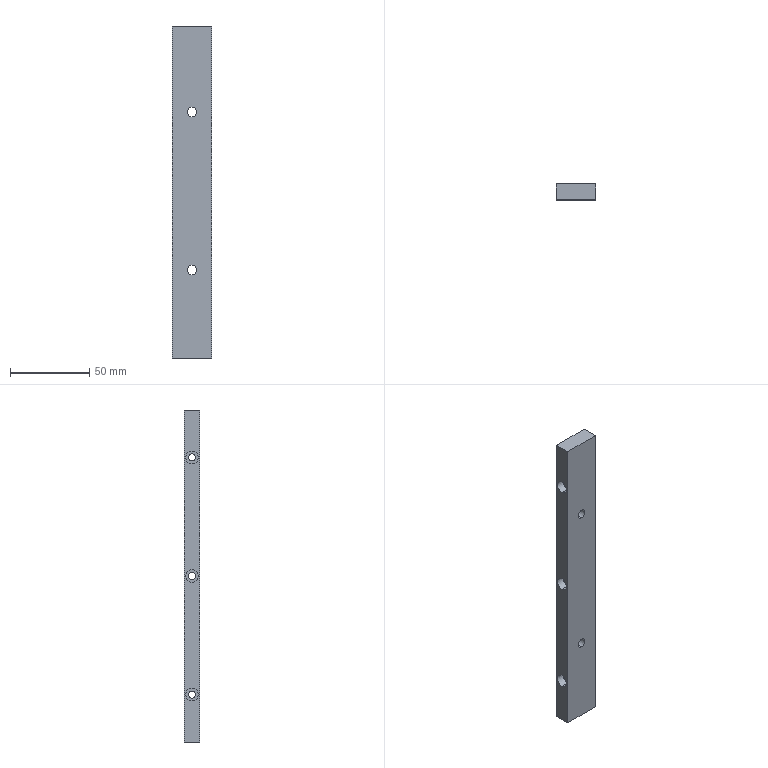Part | SolidWorks | features Extrusion 1, HoleWzd 1, ICE 1 | 1 solid | 25 faces | box 25 x 10 x 210 mm | volume 50226 mm3 | cylinder 16 | plane 9 | commonest cylinder face diameters 4.5 x6 8 x6 6 x4
STEP:
#1=CARTESIAN_POINT('',(0.,5.,-46.436));
#2=VERTEX_POINT('',#1);
#3=CARTESIAN_POINT('',(0.,5.,-52.436));
#4=VERTEX_POINT('',#3);
#5=CARTESIAN_POINT('',(0.,5.,-49.436));
#6=DIRECTION('',(0.,-1.,0.));
#7=DIRECTION('',(0.,0.,-1.));
#8=AXIS2_PLACEMENT_3D('',#5,#6,#7);
#9=CIRCLE('',#8,3.);
#10=EDGE_CURVE('',#2,#4,#9,.T.);
#11=ORIENTED_EDGE('',*,*,#10,.F.);
#12=CARTESIAN_POINT('',(0.,-5.,-46.436));
#13=VERTEX_POINT('',#12);
#14=CARTESIAN_POINT('',(0.,24.,-46.436));
#15=DIRECTION('',(0.,-1.,0.));
#16=VECTOR('',#15,1000.);
#17=LINE('',#14,#16);
#18=EDGE_CURVE('',#2,#13,#17,.T.);
#19=ORIENTED_EDGE('',*,*,#18,.T.);
#20=CARTESIAN_POINT('',(0.,-5.,-52.436));
#21=VERTEX_POINT('',#20);
#22=CARTESIAN_POINT('',(0.,-5.,-49.436));
#23=DIRECTION('',(0.,-1.,0.));
#24=DIRECTION('',(0.,0.,-1.));
#25=AXIS2_PLACEMENT_3D('',#22,#23,#24);
#26=CIRCLE('',#25,3.);
#27=EDGE_CURVE('',#13,#21,#26,.T.);
#28=ORIENTED_EDGE('',*,*,#27,.T.);
#29=CARTESIAN_POINT('',(0.,24.,-52.436));
#30=DIRECTION('',(0.,-1.,0.));
#31=VECTOR('',#30,1000.);
#32=LINE('',#29,#31);
#33=EDGE_CURVE('',#4,#21,#32,.T.);
#34=ORIENTED_EDGE('',*,*,#33,.F.);
#35=EDGE_LOOP('',(#11,#19,#28,#34));
#36=FACE_OUTER_BOUND('',#35,.T.);
#37=CARTESIAN_POINT('',(0.,24.,-49.436));
#38=DIRECTION('',(0.,-1.,0.));
#39=DIRECTION('',(0.,0.,-1.));
#40=AXIS2_PLACEMENT_3D('',#37,#38,#39);
#41=CYLINDRICAL_SURFACE('',#40,3.);
#42=ADVANCED_FACE('',(#36),#41,.F.);
#43=CARTESIAN_POINT('',(0.,5.,53.564));
#44=VERTEX_POINT('',#43);
#45=CARTESIAN_POINT('',(0.,5.,47.564));
#46=VERTEX_POINT('',#45);
#47=CARTESIAN_POINT('',(0.,5.,50.564));
#48=DIRECTION('',(0.,-1.,0.));
#49=DIRECTION('',(0.,0.,-1.));
#50=AXIS2_PLACEMENT_3D('',#47,#48,#49);
#51=CIRCLE('',#50,3.);
#52=EDGE_CURVE('',#44,#46,#51,.T.);
#53=ORIENTED_EDGE('',*,*,#52,.F.);
#54=CARTESIAN_POINT('',(0.,-5.,53.564));
#55=VERTEX_POINT('',#54);
#56=CARTESIAN_POINT('',(0.,24.,53.564));
#57=DIRECTION('',(0.,-1.,0.));
#58=VECTOR('',#57,1000.);
#59=LINE('',#56,#58);
#60=EDGE_CURVE('',#44,#55,#59,.T.);
#61=ORIENTED_EDGE('',*,*,#60,.T.);
#62=CARTESIAN_POINT('',(0.,-5.,47.564));
#63=VERTEX_POINT('',#62);
#64=CARTESIAN_POINT('',(0.,-5.,50.564));
#65=DIRECTION('',(0.,-1.,0.));
#66=DIRECTION('',(0.,0.,-1.));
#67=AXIS2_PLACEMENT_3D('',#64,#65,#66);
#68=CIRCLE('',#67,3.);
#69=EDGE_CURVE('',#55,#63,#68,.T.);
#70=ORIENTED_EDGE('',*,*,#69,.T.);
#71=CARTESIAN_POINT('',(0.,24.,47.564));
#72=DIRECTION('',(0.,-1.,0.));
#73=VECTOR('',#72,1000.);
#74=LINE('',#71,#73);
#75=EDGE_CURVE('',#46,#63,#74,.T.);
#76=ORIENTED_EDGE('',*,*,#75,.F.);
#77=EDGE_LOOP('',(#53,#61,#70,#76));
#78=FACE_OUTER_BOUND('',#77,.T.);
#79=CARTESIAN_POINT('',(0.,24.,50.564));
#80=DIRECTION('',(0.,-1.,0.));
#81=DIRECTION('',(0.,0.,-1.));
#82=AXIS2_PLACEMENT_3D('',#79,#80,#81);
#83=CYLINDRICAL_SURFACE('',#82,3.);
#84=ADVANCED_FACE('',(#78),#83,.F.);
#85=CARTESIAN_POINT('',(-7.5,0.,-4.));
#86=VERTEX_POINT('',#85);
#87=CARTESIAN_POINT('',(-7.5,0.,4.));
#88=VERTEX_POINT('',#87);
#89=CARTESIAN_POINT('',(-7.5,0.,0.));
#90=DIRECTION('',(-1.,0.,0.));
#91=DIRECTION('',(0.,0.,1.));
#92=AXIS2_PLACEMENT_3D('',#89,#90,#91);
#93=CIRCLE('',#92,4.);
#94=EDGE_CURVE('',#86,#88,#93,.T.);
#95=ORIENTED_EDGE('',*,*,#94,.F.);
#96=CARTESIAN_POINT('',(-12.5,0.,-4.));
#97=VERTEX_POINT('',#96);
#98=CARTESIAN_POINT('',(-12.5,0.,-4.));
#99=DIRECTION('',(-1.,0.,0.));
#100=VECTOR('',#99,1000.);
#101=LINE('',#98,#100);
#102=EDGE_CURVE('',#86,#97,#101,.T.);
#103=ORIENTED_EDGE('',*,*,#102,.T.);
#104=CARTESIAN_POINT('',(-12.5,0.,4.));
#105=VERTEX_POINT('',#104);
#106=CARTESIAN_POINT('',(-12.5,0.,0.));
#107=DIRECTION('',(-1.,0.,0.));
#108=DIRECTION('',(0.,0.,1.));
#109=AXIS2_PLACEMENT_3D('',#106,#107,#108);
#110=CIRCLE('',#109,4.);
#111=EDGE_CURVE('',#97,#105,#110,.T.);
#112=ORIENTED_EDGE('',*,*,#111,.T.);
#113=CARTESIAN_POINT('',(-12.5,0.,4.));
#114=DIRECTION('',(-1.,0.,0.));
#115=VECTOR('',#114,1000.);
#116=LINE('',#113,#115);
#117=EDGE_CURVE('',#88,#105,#116,.T.);
#118=ORIENTED_EDGE('',*,*,#117,.F.);
#119=EDGE_LOOP('',(#95,#103,#112,#118));
#120=FACE_OUTER_BOUND('',#119,.T.);
#121=CARTESIAN_POINT('',(-12.5,0.,0.));
#122=DIRECTION('',(-1.,0.,0.));
#123=DIRECTION('',(0.,0.,1.));
#124=AXIS2_PLACEMENT_3D('',#121,#122,#123);
#125=CYLINDRICAL_SURFACE('',#124,4.);
#126=ADVANCED_FACE('',(#120),#125,.F.);
#127=CARTESIAN_POINT('',(12.5,0.,-2.25));
#128=VERTEX_POINT('',#127);
#129=CARTESIAN_POINT('',(12.5,0.,2.25));
#130=VERTEX_POINT('',#129);
#131=CARTESIAN_POINT('',(12.5,0.,0.));
#132=DIRECTION('',(-1.,0.,0.));
#133=DIRECTION('',(0.,0.,1.));
#134=AXIS2_PLACEMENT_3D('',#131,#132,#133);
#135=CIRCLE('',#134,2.25);
#136=EDGE_CURVE('',#128,#130,#135,.T.);
#137=ORIENTED_EDGE('',*,*,#136,.F.);
#138=CARTESIAN_POINT('',(-7.5,0.,-2.25));
#139=VERTEX_POINT('',#138);
#140=CARTESIAN_POINT('',(-12.5,0.,-2.25));
#141=DIRECTION('',(-1.,0.,0.));
#142=VECTOR('',#141,1000.);
#143=LINE('',#140,#142);
#144=EDGE_CURVE('',#128,#139,#143,.T.);
#145=ORIENTED_EDGE('',*,*,#144,.T.);
#146=CARTESIAN_POINT('',(-7.5,0.,2.25));
#147=VERTEX_POINT('',#146);
#148=CARTESIAN_POINT('',(-7.5,0.,0.));
#149=DIRECTION('',(-1.,0.,0.));
#150=DIRECTION('',(0.,0.,1.));
#151=AXIS2_PLACEMENT_3D('',#148,#149,#150);
#152=CIRCLE('',#151,2.25);
#153=EDGE_CURVE('',#139,#147,#152,.T.);
#154=ORIENTED_EDGE('',*,*,#153,.T.);
#155=CARTESIAN_POINT('',(-12.5,0.,2.25));
#156=DIRECTION('',(-1.,0.,0.));
#157=VECTOR('',#156,1000.);
#158=LINE('',#155,#157);
#159=EDGE_CURVE('',#130,#147,#158,.T.);
#160=ORIENTED_EDGE('',*,*,#159,.F.);
#161=EDGE_LOOP('',(#137,#145,#154,#160));
#162=FACE_OUTER_BOUND('',#161,.T.);
#163=CARTESIAN_POINT('',(-12.5,0.,0.));
#164=DIRECTION('',(-1.,0.,0.));
#165=DIRECTION('',(0.,0.,1.));
#166=AXIS2_PLACEMENT_3D('',#163,#164,#165);
#167=CYLINDRICAL_SURFACE('',#166,2.25);
#168=ADVANCED_FACE('',(#162),#167,.F.);
#169=CARTESIAN_POINT('',(-7.5,0.,-79.));
#170=VERTEX_POINT('',#169);
#171=CARTESIAN_POINT('',(-7.5,0.,-71.));
#172=VERTEX_POINT('',#171);
#173=CARTESIAN_POINT('',(-7.5,0.,-75.));
#174=DIRECTION('',(-1.,0.,0.));
#175=DIRECTION('',(0.,0.,1.));
#176=AXIS2_PLACEMENT_3D('',#173,#174,#175);
#177=CIRCLE('',#176,4.);
#178=EDGE_CURVE('',#170,#172,#177,.T.);
#179=ORIENTED_EDGE('',*,*,#178,.F.);
#180=CARTESIAN_POINT('',(-12.5,0.,-79.));
#181=VERTEX_POINT('',#180);
#182=CARTESIAN_POINT('',(-12.5,0.,-79.));
#183=DIRECTION('',(-1.,0.,0.));
#184=VECTOR('',#183,1000.);
#185=LINE('',#182,#184);
#186=EDGE_CURVE('',#170,#181,#185,.T.);
#187=ORIENTED_EDGE('',*,*,#186,.T.);
#188=CARTESIAN_POINT('',(-12.5,0.,-71.));
#189=VERTEX_POINT('',#188);
#190=CARTESIAN_POINT('',(-12.5,0.,-75.));
#191=DIRECTION('',(-1.,0.,0.));
#192=DIRECTION('',(0.,0.,1.));
#193=AXIS2_PLACEMENT_3D('',#190,#191,#192);
#194=CIRCLE('',#193,4.);
#195=EDGE_CURVE('',#181,#189,#194,.T.);
#196=ORIENTED_EDGE('',*,*,#195,.T.);
#197=CARTESIAN_POINT('',(-12.5,0.,-71.));
#198=DIRECTION('',(-1.,0.,0.));
#199=VECTOR('',#198,1000.);
#200=LINE('',#197,#199);
#201=EDGE_CURVE('',#172,#189,#200,.T.);
#202=ORIENTED_EDGE('',*,*,#201,.F.);
#203=EDGE_LOOP('',(#179,#187,#196,#202));
#204=FACE_OUTER_BOUND('',#203,.T.);
#205=CARTESIAN_POINT('',(-12.5,0.,-75.));
#206=DIRECTION('',(-1.,0.,0.));
#207=DIRECTION('',(0.,0.,1.));
#208=AXIS2_PLACEMENT_3D('',#205,#206,#207);
#209=CYLINDRICAL_SURFACE('',#208,4.);
#210=ADVANCED_FACE('',(#204),#209,.F.);
#211=CARTESIAN_POINT('',(12.5,0.,-77.25));
#212=VERTEX_POINT('',#211);
#213=CARTESIAN_POINT('',(12.5,0.,-72.75));
#214=VERTEX_POINT('',#213);
#215=CARTESIAN_POINT('',(12.5,0.,-75.));
#216=DIRECTION('',(-1.,0.,0.));
#217=DIRECTION('',(0.,0.,1.));
#218=AXIS2_PLACEMENT_3D('',#215,#216,#217);
#219=CIRCLE('',#218,2.25);
#220=EDGE_CURVE('',#212,#214,#219,.T.);
#221=ORIENTED_EDGE('',*,*,#220,.F.);
#222=CARTESIAN_POINT('',(-7.5,0.,-77.25));
#223=VERTEX_POINT('',#222);
#224=CARTESIAN_POINT('',(-12.5,0.,-77.25));
#225=DIRECTION('',(-1.,0.,0.));
#226=VECTOR('',#225,1000.);
#227=LINE('',#224,#226);
#228=EDGE_CURVE('',#212,#223,#227,.T.);
#229=ORIENTED_EDGE('',*,*,#228,.T.);
#230=CARTESIAN_POINT('',(-7.5,0.,-72.75));
#231=VERTEX_POINT('',#230);
#232=CARTESIAN_POINT('',(-7.5,0.,-75.));
#233=DIRECTION('',(-1.,0.,0.));
#234=DIRECTION('',(0.,0.,1.));
#235=AXIS2_PLACEMENT_3D('',#232,#233,#234);
#236=CIRCLE('',#235,2.25);
#237=EDGE_CURVE('',#223,#231,#236,.T.);
#238=ORIENTED_EDGE('',*,*,#237,.T.);
#239=CARTESIAN_POINT('',(-12.5,0.,-72.75));
#240=DIRECTION('',(-1.,0.,0.));
#241=VECTOR('',#240,1000.);
#242=LINE('',#239,#241);
#243=EDGE_CURVE('',#214,#231,#242,.T.);
#244=ORIENTED_EDGE('',*,*,#243,.F.);
#245=EDGE_LOOP('',(#221,#229,#238,#244));
#246=FACE_OUTER_BOUND('',#245,.T.);
#247=CARTESIAN_POINT('',(-12.5,0.,-75.));
#248=DIRECTION('',(-1.,0.,0.));
#249=DIRECTION('',(0.,0.,1.));
#250=AXIS2_PLACEMENT_3D('',#247,#248,#249);
#251=CYLINDRICAL_SURFACE('',#250,2.25);
#252=ADVANCED_FACE('',(#246),#251,.F.);
#253=CARTESIAN_POINT('',(-7.5,0.,71.));
#254=VERTEX_POINT('',#253);
#255=CARTESIAN_POINT('',(-7.5,0.,79.));
#256=VERTEX_POINT('',#255);
#257=CARTESIAN_POINT('',(-7.5,0.,75.));
#258=DIRECTION('',(-1.,0.,0.));
#259=DIRECTION('',(0.,0.,1.));
#260=AXIS2_PLACEMENT_3D('',#257,#258,#259);
#261=CIRCLE('',#260,4.);
#262=EDGE_CURVE('',#254,#256,#261,.T.);
#263=ORIENTED_EDGE('',*,*,#262,.F.);
#264=CARTESIAN_POINT('',(-12.5,0.,71.));
#265=VERTEX_POINT('',#264);
#266=CARTESIAN_POINT('',(-12.5,0.,71.));
#267=DIRECTION('',(-1.,0.,0.));
#268=VECTOR('',#267,1000.);
#269=LINE('',#266,#268);
#270=EDGE_CURVE('',#254,#265,#269,.T.);
#271=ORIENTED_EDGE('',*,*,#270,.T.);
#272=CARTESIAN_POINT('',(-12.5,0.,79.));
#273=VERTEX_POINT('',#272);
#274=CARTESIAN_POINT('',(-12.5,0.,75.));
#275=DIRECTION('',(-1.,0.,0.));
#276=DIRECTION('',(0.,0.,1.));
#277=AXIS2_PLACEMENT_3D('',#274,#275,#276);
#278=CIRCLE('',#277,4.);
#279=EDGE_CURVE('',#265,#273,#278,.T.);
#280=ORIENTED_EDGE('',*,*,#279,.T.);
#281=CARTESIAN_POINT('',(-12.5,0.,79.));
#282=DIRECTION('',(-1.,0.,0.));
#283=VECTOR('',#282,1000.);
#284=LINE('',#281,#283);
#285=EDGE_CURVE('',#256,#273,#284,.T.);
#286=ORIENTED_EDGE('',*,*,#285,.F.);
#287=EDGE_LOOP('',(#263,#271,#280,#286));
#288=FACE_OUTER_BOUND('',#287,.T.);
#289=CARTESIAN_POINT('',(-12.5,0.,75.));
#290=DIRECTION('',(-1.,0.,0.));
#291=DIRECTION('',(0.,0.,1.));
#292=AXIS2_PLACEMENT_3D('',#289,#290,#291);
#293=CYLINDRICAL_SURFACE('',#292,4.);
#294=ADVANCED_FACE('',(#288),#293,.F.);
#295=CARTESIAN_POINT('',(12.5,0.,72.75));
#296=VERTEX_POINT('',#295);
#297=CARTESIAN_POINT('',(12.5,0.,77.25));
#298=VERTEX_POINT('',#297);
#299=CARTESIAN_POINT('',(12.5,0.,75.));
#300=DIRECTION('',(-1.,0.,0.));
#301=DIRECTION('',(0.,0.,1.));
#302=AXIS2_PLACEMENT_3D('',#299,#300,#301);
#303=CIRCLE('',#302,2.25);
#304=EDGE_CURVE('',#296,#298,#303,.T.);
#305=ORIENTED_EDGE('',*,*,#304,.F.);
#306=CARTESIAN_POINT('',(-7.5,0.,72.75));
#307=VERTEX_POINT('',#306);
#308=CARTESIAN_POINT('',(-12.5,0.,72.75));
#309=DIRECTION('',(-1.,0.,0.));
#310=VECTOR('',#309,1000.);
#311=LINE('',#308,#310);
#312=EDGE_CURVE('',#296,#307,#311,.T.);
#313=ORIENTED_EDGE('',*,*,#312,.T.);
#314=CARTESIAN_POINT('',(-7.5,0.,77.25));
#315=VERTEX_POINT('',#314);
#316=CARTESIAN_POINT('',(-7.5,0.,75.));
#317=DIRECTION('',(-1.,0.,0.));
#318=DIRECTION('',(0.,0.,1.));
#319=AXIS2_PLACEMENT_3D('',#316,#317,#318);
#320=CIRCLE('',#319,2.25);
#321=EDGE_CURVE('',#307,#315,#320,.T.);
#322=ORIENTED_EDGE('',*,*,#321,.T.);
#323=CARTESIAN_POINT('',(-12.5,0.,77.25));
#324=DIRECTION('',(-1.,0.,0.));
#325=VECTOR('',#324,1000.);
#326=LINE('',#323,#325);
#327=EDGE_CURVE('',#298,#315,#326,.T.);
#328=ORIENTED_EDGE('',*,*,#327,.F.);
#329=EDGE_LOOP('',(#305,#313,#322,#328));
#330=FACE_OUTER_BOUND('',#329,.T.);
#331=CARTESIAN_POINT('',(-12.5,0.,75.));
#332=DIRECTION('',(-1.,0.,0.));
#333=DIRECTION('',(0.,0.,1.));
#334=AXIS2_PLACEMENT_3D('',#331,#332,#333);
#335=CYLINDRICAL_SURFACE('',#334,2.25);
#336=ADVANCED_FACE('',(#330),#335,.F.);
#337=CARTESIAN_POINT('',(-12.5,-5.,-105.));
#338=VERTEX_POINT('',#337);
#339=CARTESIAN_POINT('',(-12.5,5.,-105.));
#340=VERTEX_POINT('',#339);
#341=CARTESIAN_POINT('',(-12.5,5.,-105.));
#342=DIRECTION('',(0.,1.,0.));
#343=VECTOR('',#342,1000.);
#344=LINE('',#341,#343);
#345=EDGE_CURVE('',#338,#340,#344,.T.);
#346=ORIENTED_EDGE('',*,*,#345,.T.);
#347=CARTESIAN_POINT('',(12.5,5.,-105.));
#348=VERTEX_POINT('',#347);
#349=CARTESIAN_POINT('',(12.5,5.,-105.));
#350=DIRECTION('',(-1.,0.,0.));
#351=VECTOR('',#350,1000.);
#352=LINE('',#349,#351);
#353=EDGE_CURVE('',#348,#340,#352,.T.);
#354=ORIENTED_EDGE('',*,*,#353,.F.);
#355=CARTESIAN_POINT('',(12.5,-5.,-105.));
#356=VERTEX_POINT('',#355);
#357=CARTESIAN_POINT('',(12.5,5.,-105.));
#358=DIRECTION('',(0.,1.,0.));
#359=VECTOR('',#358,1000.);
#360=LINE('',#357,#359);
#361=EDGE_CURVE('',#356,#348,#360,.T.);
#362=ORIENTED_EDGE('',*,*,#361,.F.);
#363=CARTESIAN_POINT('',(12.5,-5.,-105.));
#364=DIRECTION('',(-1.,0.,0.));
#365=VECTOR('',#364,1000.);
#366=LINE('',#363,#365);
#367=EDGE_CURVE('',#356,#338,#366,.T.);
#368=ORIENTED_EDGE('',*,*,#367,.T.);
#369=EDGE_LOOP('',(#346,#354,#362,#368));
#370=FACE_OUTER_BOUND('',#369,.T.);
#371=CARTESIAN_POINT('',(12.5,5.,-105.));
#372=DIRECTION('',(0.,0.,1.));
#373=DIRECTION('',(1.,0.,0.));
#374=AXIS2_PLACEMENT_3D('',#371,#372,#373);
#375=PLANE('',#374);
#376=ADVANCED_FACE('',(#370),#375,.F.);
#377=CARTESIAN_POINT('',(0.,5.,-49.436));
#378=DIRECTION('',(0.,-1.,0.));
#379=DIRECTION('',(0.,0.,-1.));
#380=AXIS2_PLACEMENT_3D('',#377,#378,#379);
#381=CIRCLE('',#380,3.);
#382=EDGE_CURVE('',#4,#2,#381,.T.);
#383=ORIENTED_EDGE('',*,*,#382,.T.);
#384=ORIENTED_EDGE('',*,*,#10,.T.);
#385=EDGE_LOOP('',(#383,#384));
#386=FACE_BOUND('',#385,.T.);
#387=CARTESIAN_POINT('',(0.,5.,50.564));
#388=DIRECTION('',(0.,-1.,0.));
#389=DIRECTION('',(0.,0.,-1.));
#390=AXIS2_PLACEMENT_3D('',#387,#388,#389);
#391=CIRCLE('',#390,3.);
#392=EDGE_CURVE('',#46,#44,#391,.T.);
#393=ORIENTED_EDGE('',*,*,#392,.T.);
#394=ORIENTED_EDGE('',*,*,#52,.T.);
#395=EDGE_LOOP('',(#393,#394));
#396=FACE_BOUND('',#395,.T.);
#397=CARTESIAN_POINT('',(-12.5,5.,105.));
#398=VERTEX_POINT('',#397);
#399=CARTESIAN_POINT('',(-12.5,5.,105.));
#400=DIRECTION('',(0.,0.,1.));
#401=VECTOR('',#400,1000.);
#402=LINE('',#399,#401);
#403=EDGE_CURVE('',#340,#398,#402,.T.);
#404=ORIENTED_EDGE('',*,*,#403,.T.);
#405=CARTESIAN_POINT('',(12.5,5.,105.));
#406=VERTEX_POINT('',#405);
#407=CARTESIAN_POINT('',(12.5,5.,105.));
#408=DIRECTION('',(-1.,0.,0.));
#409=VECTOR('',#408,1000.);
#410=LINE('',#407,#409);
#411=EDGE_CURVE('',#406,#398,#410,.T.);
#412=ORIENTED_EDGE('',*,*,#411,.F.);
#413=CARTESIAN_POINT('',(12.5,5.,105.));
#414=DIRECTION('',(0.,0.,1.));
#415=VECTOR('',#414,1000.);
#416=LINE('',#413,#415);
#417=EDGE_CURVE('',#348,#406,#416,.T.);
#418=ORIENTED_EDGE('',*,*,#417,.F.);
#419=ORIENTED_EDGE('',*,*,#353,.T.);
#420=EDGE_LOOP('',(#404,#412,#418,#419));
#421=FACE_OUTER_BOUND('',#420,.T.);
#422=CARTESIAN_POINT('',(12.5,5.,105.));
#423=DIRECTION('',(0.,-1.,0.));
#424=DIRECTION('',(0.,0.,-1.));
#425=AXIS2_PLACEMENT_3D('',#422,#423,#424);
#426=PLANE('',#425);
#427=ADVANCED_FACE('',(#386,#396,#421),#426,.F.);
#428=CARTESIAN_POINT('',(-12.5,-5.,105.));
#429=VERTEX_POINT('',#428);
#430=CARTESIAN_POINT('',(-12.5,5.,105.));
#431=DIRECTION('',(0.,-1.,0.));
#432=VECTOR('',#431,1000.);
#433=LINE('',#430,#432);
#434=EDGE_CURVE('',#398,#429,#433,.T.);
#435=ORIENTED_EDGE('',*,*,#434,.T.);
#436=CARTESIAN_POINT('',(12.5,-5.,105.));
#437=VERTEX_POINT('',#436);
#438=CARTESIAN_POINT('',(12.5,-5.,105.));
#439=DIRECTION('',(-1.,0.,0.));
#440=VECTOR('',#439,1000.);
#441=LINE('',#438,#440);
#442=EDGE_CURVE('',#437,#429,#441,.T.);
#443=ORIENTED_EDGE('',*,*,#442,.F.);
#444=CARTESIAN_POINT('',(12.5,5.,105.));
#445=DIRECTION('',(0.,-1.,0.));
#446=VECTOR('',#445,1000.);
#447=LINE('',#444,#446);
#448=EDGE_CURVE('',#406,#437,#447,.T.);
#449=ORIENTED_EDGE('',*,*,#448,.F.);
#450=ORIENTED_EDGE('',*,*,#411,.T.);
#451=EDGE_LOOP('',(#435,#443,#449,#450));
#452=FACE_OUTER_BOUND('',#451,.T.);
#453=CARTESIAN_POINT('',(12.5,5.,105.));
#454=DIRECTION('',(0.,0.,-1.));
#455=DIRECTION('',(-1.,0.,0.));
#456=AXIS2_PLACEMENT_3D('',#453,#454,#455);
#457=PLANE('',#456);
#458=ADVANCED_FACE('',(#452),#457,.F.);
#459=CARTESIAN_POINT('',(0.,-5.,-49.436));
#460=DIRECTION('',(0.,-1.,0.));
#461=DIRECTION('',(0.,0.,-1.));
#462=AXIS2_PLACEMENT_3D('',#459,#460,#461);
#463=CIRCLE('',#462,3.);
#464=EDGE_CURVE('',#21,#13,#463,.T.);
#465=ORIENTED_EDGE('',*,*,#464,.F.);
#466=ORIENTED_EDGE('',*,*,#27,.F.);
#467=EDGE_LOOP('',(#465,#466));
#468=FACE_BOUND('',#467,.T.);
#469=CARTESIAN_POINT('',(0.,-5.,50.564));
#470=DIRECTION('',(0.,-1.,0.));
#471=DIRECTION('',(0.,0.,-1.));
#472=AXIS2_PLACEMENT_3D('',#469,#470,#471);
#473=CIRCLE('',#472,3.);
#474=EDGE_CURVE('',#63,#55,#473,.T.);
#475=ORIENTED_EDGE('',*,*,#474,.F.);
#476=ORIENTED_EDGE('',*,*,#69,.F.);
#477=EDGE_LOOP('',(#475,#476));
#478=FACE_BOUND('',#477,.T.);
#479=CARTESIAN_POINT('',(-12.5,-5.,105.));
#480=DIRECTION('',(0.,0.,-1.));
#481=VECTOR('',#480,1000.);
#482=LINE('',#479,#481);
#483=EDGE_CURVE('',#429,#338,#482,.T.);
#484=ORIENTED_EDGE('',*,*,#483,.T.);
#485=ORIENTED_EDGE('',*,*,#367,.F.);
#486=CARTESIAN_POINT('',(12.5,-5.,105.));
#487=DIRECTION('',(0.,0.,-1.));
#488=VECTOR('',#487,1000.);
#489=LINE('',#486,#488);
#490=EDGE_CURVE('',#437,#356,#489,.T.);
#491=ORIENTED_EDGE('',*,*,#490,.F.);
#492=ORIENTED_EDGE('',*,*,#442,.T.);
#493=EDGE_LOOP('',(#484,#485,#491,#492));
#494=FACE_OUTER_BOUND('',#493,.T.);
#495=CARTESIAN_POINT('',(12.5,-5.,105.));
#496=DIRECTION('',(0.,1.,0.));
#497=DIRECTION('',(0.,0.,1.));
#498=AXIS2_PLACEMENT_3D('',#495,#496,#497);
#499=PLANE('',#498);
#500=ADVANCED_FACE('',(#468,#478,#494),#499,.F.);
#501=CARTESIAN_POINT('',(12.5,0.,0.));
#502=DIRECTION('',(-1.,0.,0.));
#503=DIRECTION('',(0.,0.,1.));
#504=AXIS2_PLACEMENT_3D('',#501,#502,#503);
#505=CIRCLE('',#504,2.25);
#506=EDGE_CURVE('',#130,#128,#505,.T.);
#507=ORIENTED_EDGE('',*,*,#506,.T.);
#508=ORIENTED_EDGE('',*,*,#136,.T.);
#509=EDGE_LOOP('',(#507,#508));
#510=FACE_BOUND('',#509,.T.);
#511=CARTESIAN_POINT('',(12.5,0.,-75.));
#512=DIRECTION('',(-1.,0.,0.));
#513=DIRECTION('',(0.,0.,1.));
#514=AXIS2_PLACEMENT_3D('',#511,#512,#513);
#515=CIRCLE('',#514,2.25);
#516=EDGE_CURVE('',#214,#212,#515,.T.);
#517=ORIENTED_EDGE('',*,*,#516,.T.);
#518=ORIENTED_EDGE('',*,*,#220,.T.);
#519=EDGE_LOOP('',(#517,#518));
#520=FACE_BOUND('',#519,.T.);
#521=CARTESIAN_POINT('',(12.5,0.,75.));
#522=DIRECTION('',(-1.,0.,0.));
#523=DIRECTION('',(0.,0.,1.));
#524=AXIS2_PLACEMENT_3D('',#521,#522,#523);
#525=CIRCLE('',#524,2.25);
#526=EDGE_CURVE('',#298,#296,#525,.T.);
#527=ORIENTED_EDGE('',*,*,#526,.T.);
#528=ORIENTED_EDGE('',*,*,#304,.T.);
#529=EDGE_LOOP('',(#527,#528));
#530=FACE_BOUND('',#529,.T.);
#531=ORIENTED_EDGE('',*,*,#361,.T.);
#532=ORIENTED_EDGE('',*,*,#417,.T.);
#533=ORIENTED_EDGE('',*,*,#448,.T.);
#534=ORIENTED_EDGE('',*,*,#490,.T.);
#535=EDGE_LOOP('',(#531,#532,#533,#534));
#536=FACE_OUTER_BOUND('',#535,.T.);
#537=CARTESIAN_POINT('',(12.5,0.,0.));
#538=DIRECTION('',(1.,0.,0.));
#539=DIRECTION('',(0.,0.,-1.));
#540=AXIS2_PLACEMENT_3D('',#537,#538,#539);
#541=PLANE('',#540);
#542=ADVANCED_FACE('',(#510,#520,#530,#536),#541,.T.);
#543=CARTESIAN_POINT('',(-12.5,0.,0.));
#544=DIRECTION('',(-1.,0.,0.));
#545=DIRECTION('',(0.,0.,1.));
#546=AXIS2_PLACEMENT_3D('',#543,#544,#545);
#547=CIRCLE('',#546,4.);
#548=EDGE_CURVE('',#105,#97,#547,.T.);
#549=ORIENTED_EDGE('',*,*,#548,.F.);
#550=ORIENTED_EDGE('',*,*,#111,.F.);
#551=EDGE_LOOP('',(#549,#550));
#552=FACE_BOUND('',#551,.T.);
#553=CARTESIAN_POINT('',(-12.5,0.,-75.));
#554=DIRECTION('',(-1.,0.,0.));
#555=DIRECTION('',(0.,0.,1.));
#556=AXIS2_PLACEMENT_3D('',#553,#554,#555);
#557=CIRCLE('',#556,4.);
#558=EDGE_CURVE('',#189,#181,#557,.T.);
#559=ORIENTED_EDGE('',*,*,#558,.F.);
#560=ORIENTED_EDGE('',*,*,#195,.F.);
#561=EDGE_LOOP('',(#559,#560));
#562=FACE_BOUND('',#561,.T.);
#563=CARTESIAN_POINT('',(-12.5,0.,75.));
#564=DIRECTION('',(-1.,0.,0.));
#565=DIRECTION('',(0.,0.,1.));
#566=AXIS2_PLACEMENT_3D('',#563,#564,#565);
#567=CIRCLE('',#566,4.);
#568=EDGE_CURVE('',#273,#265,#567,.T.);
#569=ORIENTED_EDGE('',*,*,#568,.F.);
#570=ORIENTED_EDGE('',*,*,#279,.F.);
#571=EDGE_LOOP('',(#569,#570));
#572=FACE_BOUND('',#571,.T.);
#573=ORIENTED_EDGE('',*,*,#345,.F.);
#574=ORIENTED_EDGE('',*,*,#483,.F.);
#575=ORIENTED_EDGE('',*,*,#434,.F.);
#576=ORIENTED_EDGE('',*,*,#403,.F.);
#577=EDGE_LOOP('',(#573,#574,#575,#576));
#578=FACE_OUTER_BOUND('',#577,.T.);
#579=CARTESIAN_POINT('',(-12.5,0.,0.));
#580=DIRECTION('',(1.,0.,0.));
#581=DIRECTION('',(0.,0.,-1.));
#582=AXIS2_PLACEMENT_3D('',#579,#580,#581);
#583=PLANE('',#582);
#584=ADVANCED_FACE('',(#552,#562,#572,#578),#583,.F.);
#585=ORIENTED_EDGE('',*,*,#312,.F.);
#586=ORIENTED_EDGE('',*,*,#526,.F.);
#587=ORIENTED_EDGE('',*,*,#327,.T.);
#588=CARTESIAN_POINT('',(-7.5,0.,75.));
#589=DIRECTION('',(-1.,0.,0.));
#590=DIRECTION('',(0.,0.,1.));
#591=AXIS2_PLACEMENT_3D('',#588,#589,#590);
#592=CIRCLE('',#591,2.25);
#593=EDGE_CURVE('',#315,#307,#592,.T.);
#594=ORIENTED_EDGE('',*,*,#593,.T.);
#595=EDGE_LOOP('',(#585,#586,#587,#594));
#596=FACE_OUTER_BOUND('',#595,.T.);
#597=CARTESIAN_POINT('',(-12.5,0.,75.));
#598=DIRECTION('',(-1.,0.,0.));
#599=DIRECTION('',(0.,0.,1.));
#600=AXIS2_PLACEMENT_3D('',#597,#598,#599);
#601=CYLINDRICAL_SURFACE('',#600,2.25);
#602=ADVANCED_FACE('',(#596),#601,.F.);
#603=ORIENTED_EDGE('',*,*,#593,.F.);
#604=ORIENTED_EDGE('',*,*,#321,.F.);
#605=EDGE_LOOP('',(#603,#604));
#606=FACE_BOUND('',#605,.T.);
#607=CARTESIAN_POINT('',(-7.5,0.,75.));
#608=DIRECTION('',(-1.,0.,0.));
#609=DIRECTION('',(0.,0.,1.));
#610=AXIS2_PLACEMENT_3D('',#607,#608,#609);
#611=CIRCLE('',#610,4.);
#612=EDGE_CURVE('',#256,#254,#611,.T.);
#613=ORIENTED_EDGE('',*,*,#612,.T.);
#614=ORIENTED_EDGE('',*,*,#262,.T.);
#615=EDGE_LOOP('',(#613,#614));
#616=FACE_OUTER_BOUND('',#615,.T.);
#617=CARTESIAN_POINT('',(-7.5,2.25,75.));
#618=DIRECTION('',(1.,0.,0.));
#619=DIRECTION('',(0.,0.,-1.));
#620=AXIS2_PLACEMENT_3D('',#617,#618,#619);
#621=PLANE('',#620);
#622=ADVANCED_FACE('',(#606,#616),#621,.F.);
#623=ORIENTED_EDGE('',*,*,#270,.F.);
#624=ORIENTED_EDGE('',*,*,#612,.F.);
#625=ORIENTED_EDGE('',*,*,#285,.T.);
#626=ORIENTED_EDGE('',*,*,#568,.T.);
#627=EDGE_LOOP('',(#623,#624,#625,#626));
#628=FACE_OUTER_BOUND('',#627,.T.);
#629=CARTESIAN_POINT('',(-12.5,0.,75.));
#630=DIRECTION('',(-1.,0.,0.));
#631=DIRECTION('',(0.,0.,1.));
#632=AXIS2_PLACEMENT_3D('',#629,#630,#631);
#633=CYLINDRICAL_SURFACE('',#632,4.);
#634=ADVANCED_FACE('',(#628),#633,.F.);
#635=ORIENTED_EDGE('',*,*,#228,.F.);
#636=ORIENTED_EDGE('',*,*,#516,.F.);
#637=ORIENTED_EDGE('',*,*,#243,.T.);
#638=CARTESIAN_POINT('',(-7.5,0.,-75.));
#639=DIRECTION('',(-1.,0.,0.));
#640=DIRECTION('',(0.,0.,1.));
#641=AXIS2_PLACEMENT_3D('',#638,#639,#640);
#642=CIRCLE('',#641,2.25);
#643=EDGE_CURVE('',#231,#223,#642,.T.);
#644=ORIENTED_EDGE('',*,*,#643,.T.);
#645=EDGE_LOOP('',(#635,#636,#637,#644));
#646=FACE_OUTER_BOUND('',#645,.T.);
#647=CARTESIAN_POINT('',(-12.5,0.,-75.));
#648=DIRECTION('',(-1.,0.,0.));
#649=DIRECTION('',(0.,0.,1.));
#650=AXIS2_PLACEMENT_3D('',#647,#648,#649);
#651=CYLINDRICAL_SURFACE('',#650,2.25);
#652=ADVANCED_FACE('',(#646),#651,.F.);
#653=ORIENTED_EDGE('',*,*,#643,.F.);
#654=ORIENTED_EDGE('',*,*,#237,.F.);
#655=EDGE_LOOP('',(#653,#654));
#656=FACE_BOUND('',#655,.T.);
#657=CARTESIAN_POINT('',(-7.5,0.,-75.));
#658=DIRECTION('',(-1.,0.,0.));
#659=DIRECTION('',(0.,0.,1.));
#660=AXIS2_PLACEMENT_3D('',#657,#658,#659);
#661=CIRCLE('',#660,4.);
#662=EDGE_CURVE('',#172,#170,#661,.T.);
#663=ORIENTED_EDGE('',*,*,#662,.T.);
#664=ORIENTED_EDGE('',*,*,#178,.T.);
#665=EDGE_LOOP('',(#663,#664));
#666=FACE_OUTER_BOUND('',#665,.T.);
#667=CARTESIAN_POINT('',(-7.5,2.25,-75.));
#668=DIRECTION('',(1.,0.,0.));
#669=DIRECTION('',(0.,0.,-1.));
#670=AXIS2_PLACEMENT_3D('',#667,#668,#669);
#671=PLANE('',#670);
#672=ADVANCED_FACE('',(#656,#666),#671,.F.);
#673=ORIENTED_EDGE('',*,*,#186,.F.);
#674=ORIENTED_EDGE('',*,*,#662,.F.);
#675=ORIENTED_EDGE('',*,*,#201,.T.);
#676=ORIENTED_EDGE('',*,*,#558,.T.);
#677=EDGE_LOOP('',(#673,#674,#675,#676));
#678=FACE_OUTER_BOUND('',#677,.T.);
#679=CARTESIAN_POINT('',(-12.5,0.,-75.));
#680=DIRECTION('',(-1.,0.,0.));
#681=DIRECTION('',(0.,0.,1.));
#682=AXIS2_PLACEMENT_3D('',#679,#680,#681);
#683=CYLINDRICAL_SURFACE('',#682,4.);
#684=ADVANCED_FACE('',(#678),#683,.F.);
#685=ORIENTED_EDGE('',*,*,#144,.F.);
#686=ORIENTED_EDGE('',*,*,#506,.F.);
#687=ORIENTED_EDGE('',*,*,#159,.T.);
#688=CARTESIAN_POINT('',(-7.5,0.,0.));
#689=DIRECTION('',(-1.,0.,0.));
#690=DIRECTION('',(0.,0.,1.));
#691=AXIS2_PLACEMENT_3D('',#688,#689,#690);
#692=CIRCLE('',#691,2.25);
#693=EDGE_CURVE('',#147,#139,#692,.T.);
#694=ORIENTED_EDGE('',*,*,#693,.T.);
#695=EDGE_LOOP('',(#685,#686,#687,#694));
#696=FACE_OUTER_BOUND('',#695,.T.);
#697=CARTESIAN_POINT('',(-12.5,0.,0.));
#698=DIRECTION('',(-1.,0.,0.));
#699=DIRECTION('',(0.,0.,1.));
#700=AXIS2_PLACEMENT_3D('',#697,#698,#699);
#701=CYLINDRICAL_SURFACE('',#700,2.25);
#702=ADVANCED_FACE('',(#696),#701,.F.);
#703=ORIENTED_EDGE('',*,*,#693,.F.);
#704=ORIENTED_EDGE('',*,*,#153,.F.);
#705=EDGE_LOOP('',(#703,#704));
#706=FACE_BOUND('',#705,.T.);
#707=CARTESIAN_POINT('',(-7.5,0.,0.));
#708=DIRECTION('',(-1.,0.,0.));
#709=DIRECTION('',(0.,0.,1.));
#710=AXIS2_PLACEMENT_3D('',#707,#708,#709);
#711=CIRCLE('',#710,4.);
#712=EDGE_CURVE('',#88,#86,#711,.T.);
#713=ORIENTED_EDGE('',*,*,#712,.T.);
#714=ORIENTED_EDGE('',*,*,#94,.T.);
#715=EDGE_LOOP('',(#713,#714));
#716=FACE_OUTER_BOUND('',#715,.T.);
#717=CARTESIAN_POINT('',(-7.5,2.25,0.));
#718=DIRECTION('',(1.,0.,0.));
#719=DIRECTION('',(0.,0.,-1.));
#720=AXIS2_PLACEMENT_3D('',#717,#718,#719);
#721=PLANE('',#720);
#722=ADVANCED_FACE('',(#706,#716),#721,.F.);
#723=ORIENTED_EDGE('',*,*,#102,.F.);
#724=ORIENTED_EDGE('',*,*,#712,.F.);
#725=ORIENTED_EDGE('',*,*,#117,.T.);
#726=ORIENTED_EDGE('',*,*,#548,.T.);
#727=EDGE_LOOP('',(#723,#724,#725,#726));
#728=FACE_OUTER_BOUND('',#727,.T.);
#729=CARTESIAN_POINT('',(-12.5,0.,0.));
#730=DIRECTION('',(-1.,0.,0.));
#731=DIRECTION('',(0.,0.,1.));
#732=AXIS2_PLACEMENT_3D('',#729,#730,#731);
#733=CYLINDRICAL_SURFACE('',#732,4.);
#734=ADVANCED_FACE('',(#728),#733,.F.);
#735=ORIENTED_EDGE('',*,*,#60,.F.);
#736=ORIENTED_EDGE('',*,*,#392,.F.);
#737=ORIENTED_EDGE('',*,*,#75,.T.);
#738=ORIENTED_EDGE('',*,*,#474,.T.);
#739=EDGE_LOOP('',(#735,#736,#737,#738));
#740=FACE_OUTER_BOUND('',#739,.T.);
#741=CARTESIAN_POINT('',(0.,24.,50.564));
#742=DIRECTION('',(0.,-1.,0.));
#743=DIRECTION('',(0.,0.,-1.));
#744=AXIS2_PLACEMENT_3D('',#741,#742,#743);
#745=CYLINDRICAL_SURFACE('',#744,3.);
#746=ADVANCED_FACE('',(#740),#745,.F.);
#747=ORIENTED_EDGE('',*,*,#18,.F.);
#748=ORIENTED_EDGE('',*,*,#382,.F.);
#749=ORIENTED_EDGE('',*,*,#33,.T.);
#750=ORIENTED_EDGE('',*,*,#464,.T.);
#751=EDGE_LOOP('',(#747,#748,#749,#750));
#752=FACE_OUTER_BOUND('',#751,.T.);
#753=CARTESIAN_POINT('',(0.,24.,-49.436));
#754=DIRECTION('',(0.,-1.,0.));
#755=DIRECTION('',(0.,0.,-1.));
#756=AXIS2_PLACEMENT_3D('',#753,#754,#755);
#757=CYLINDRICAL_SURFACE('',#756,3.);
#758=ADVANCED_FACE('',(#752),#757,.F.);
#759=CLOSED_SHELL('',(#42,#84,#126,#168,#210,#252,#294,#336,#376,#427,#458,#500,#542,#584,#602,#622,#634,#652,#672,#684,#702,#722,#734,#746,#758));
#760=MANIFOLD_SOLID_BREP('',#759);
#761=CARTESIAN_POINT('',(0.,0.,0.));
#762=DIRECTION('',(0.,0.,1.));
#763=DIRECTION('',(1.,0.,0.));
#764=AXIS2_PLACEMENT_3D('',#761,#762,#763);
#765=(LENGTH_UNIT()NAMED_UNIT(*)SI_UNIT(.MILLI.,.METRE.));
#766=UNCERTAINTY_MEASURE_WITH_UNIT(LENGTH_MEASURE(0.00001),#765,'','');
#767=(NAMED_UNIT(*)PLANE_ANGLE_UNIT()SI_UNIT($,.RADIAN.));
#768=(NAMED_UNIT(*)SI_UNIT($,.STERADIAN.)SOLID_ANGLE_UNIT());
#769=(GEOMETRIC_REPRESENTATION_CONTEXT(3)GLOBAL_UNCERTAINTY_ASSIGNED_CONTEXT((#766))GLOBAL_UNIT_ASSIGNED_CONTEXT((#765,#767,#768))REPRESENTATION_CONTEXT('',''));
#770=ADVANCED_BREP_SHAPE_REPRESENTATION('',(#760,#764),#769);